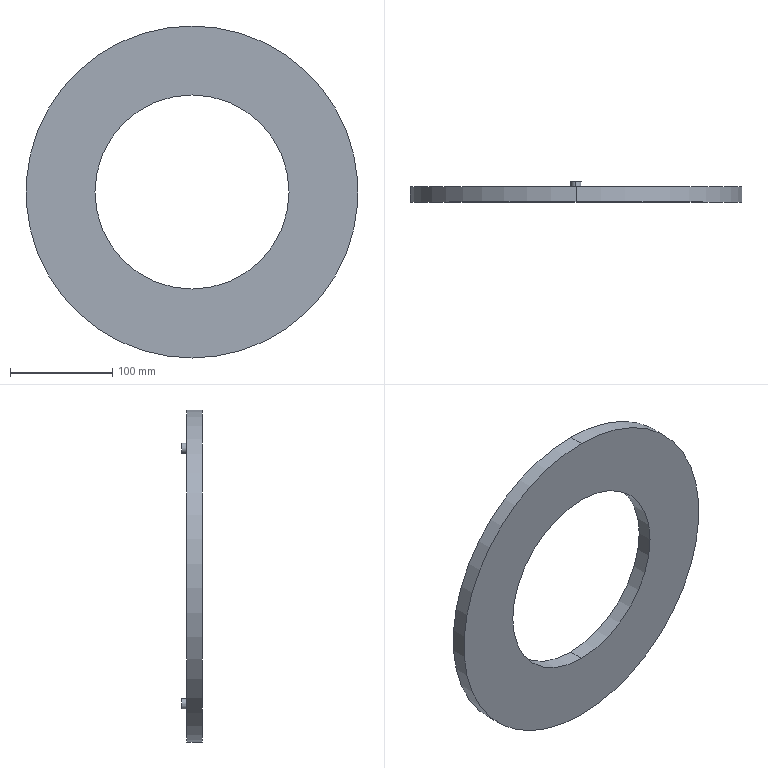Part | SolidWorks | features BaseBody 1 | 1 solid | 12 faces | box 325 x 20 x 325 mm | volume 819858 mm3 | cylinder 8 | plane 4 | commonest cylinder face diameters 10 x4 190 x2 325 x2
STEP:
#1=CARTESIAN_POINT('',(0.,20.,-120.));
#2=VERTEX_POINT('',#1);
#3=CARTESIAN_POINT('',(0.,20.,-130.));
#4=VERTEX_POINT('',#3);
#5=CARTESIAN_POINT('',(0.,20.,-125.));
#6=DIRECTION('',(0.,1.,0.));
#7=DIRECTION('',(0.,0.,1.));
#8=AXIS2_PLACEMENT_3D('',#5,#6,#7);
#9=CIRCLE('',#8,5.);
#10=EDGE_CURVE('',#2,#4,#9,.T.);
#11=ORIENTED_EDGE('',*,*,#10,.F.);
#12=CARTESIAN_POINT('',(0.,15.,-120.));
#13=VERTEX_POINT('',#12);
#14=CARTESIAN_POINT('',(0.,20.,-120.));
#15=DIRECTION('',(0.,-1.,0.));
#16=VECTOR('',#15,1000.);
#17=LINE('',#14,#16);
#18=EDGE_CURVE('',#2,#13,#17,.T.);
#19=ORIENTED_EDGE('',*,*,#18,.T.);
#20=CARTESIAN_POINT('',(0.,15.,-130.));
#21=VERTEX_POINT('',#20);
#22=CARTESIAN_POINT('',(0.,15.,-125.));
#23=DIRECTION('',(0.,1.,0.));
#24=DIRECTION('',(0.,0.,1.));
#25=AXIS2_PLACEMENT_3D('',#22,#23,#24);
#26=CIRCLE('',#25,5.);
#27=EDGE_CURVE('',#13,#21,#26,.T.);
#28=ORIENTED_EDGE('',*,*,#27,.T.);
#29=CARTESIAN_POINT('',(0.,20.,-130.));
#30=DIRECTION('',(0.,-1.,0.));
#31=VECTOR('',#30,1000.);
#32=LINE('',#29,#31);
#33=EDGE_CURVE('',#4,#21,#32,.T.);
#34=ORIENTED_EDGE('',*,*,#33,.F.);
#35=EDGE_LOOP('',(#11,#19,#28,#34));
#36=FACE_OUTER_BOUND('',#35,.T.);
#37=CARTESIAN_POINT('',(0.,20.,-125.));
#38=DIRECTION('',(0.,-1.,0.));
#39=DIRECTION('',(0.,0.,-1.));
#40=AXIS2_PLACEMENT_3D('',#37,#38,#39);
#41=CYLINDRICAL_SURFACE('',#40,5.);
#42=ADVANCED_FACE('',(#36),#41,.T.);
#43=CARTESIAN_POINT('',(0.,20.,130.));
#44=VERTEX_POINT('',#43);
#45=CARTESIAN_POINT('',(0.,20.,120.));
#46=VERTEX_POINT('',#45);
#47=CARTESIAN_POINT('',(0.,20.,125.));
#48=DIRECTION('',(0.,1.,0.));
#49=DIRECTION('',(0.,0.,1.));
#50=AXIS2_PLACEMENT_3D('',#47,#48,#49);
#51=CIRCLE('',#50,5.);
#52=EDGE_CURVE('',#44,#46,#51,.T.);
#53=ORIENTED_EDGE('',*,*,#52,.F.);
#54=CARTESIAN_POINT('',(0.,15.,130.));
#55=VERTEX_POINT('',#54);
#56=CARTESIAN_POINT('',(0.,20.,130.));
#57=DIRECTION('',(0.,-1.,0.));
#58=VECTOR('',#57,1000.);
#59=LINE('',#56,#58);
#60=EDGE_CURVE('',#44,#55,#59,.T.);
#61=ORIENTED_EDGE('',*,*,#60,.T.);
#62=CARTESIAN_POINT('',(0.,15.,120.));
#63=VERTEX_POINT('',#62);
#64=CARTESIAN_POINT('',(0.,15.,125.));
#65=DIRECTION('',(0.,1.,0.));
#66=DIRECTION('',(0.,0.,1.));
#67=AXIS2_PLACEMENT_3D('',#64,#65,#66);
#68=CIRCLE('',#67,5.);
#69=EDGE_CURVE('',#55,#63,#68,.T.);
#70=ORIENTED_EDGE('',*,*,#69,.T.);
#71=CARTESIAN_POINT('',(0.,20.,120.));
#72=DIRECTION('',(0.,-1.,0.));
#73=VECTOR('',#72,1000.);
#74=LINE('',#71,#73);
#75=EDGE_CURVE('',#46,#63,#74,.T.);
#76=ORIENTED_EDGE('',*,*,#75,.F.);
#77=EDGE_LOOP('',(#53,#61,#70,#76));
#78=FACE_OUTER_BOUND('',#77,.T.);
#79=CARTESIAN_POINT('',(0.,20.,125.));
#80=DIRECTION('',(0.,-1.,0.));
#81=DIRECTION('',(0.,0.,-1.));
#82=AXIS2_PLACEMENT_3D('',#79,#80,#81);
#83=CYLINDRICAL_SURFACE('',#82,5.);
#84=ADVANCED_FACE('',(#78),#83,.T.);
#85=CARTESIAN_POINT('',(0.,0.,-95.));
#86=VERTEX_POINT('',#85);
#87=CARTESIAN_POINT('',(0.,0.,95.));
#88=VERTEX_POINT('',#87);
#89=CARTESIAN_POINT('',(0.,0.,0.));
#90=DIRECTION('',(0.,1.,0.));
#91=DIRECTION('',(0.,0.,1.));
#92=AXIS2_PLACEMENT_3D('',#89,#90,#91);
#93=CIRCLE('',#92,95.);
#94=EDGE_CURVE('',#86,#88,#93,.T.);
#95=ORIENTED_EDGE('',*,*,#94,.F.);
#96=CARTESIAN_POINT('',(0.,15.,-95.));
#97=VERTEX_POINT('',#96);
#98=CARTESIAN_POINT('',(0.,0.,-95.));
#99=DIRECTION('',(0.,1.,0.));
#100=VECTOR('',#99,1000.);
#101=LINE('',#98,#100);
#102=EDGE_CURVE('',#86,#97,#101,.T.);
#103=ORIENTED_EDGE('',*,*,#102,.T.);
#104=CARTESIAN_POINT('',(0.,15.,95.));
#105=VERTEX_POINT('',#104);
#106=CARTESIAN_POINT('',(0.,15.,0.));
#107=DIRECTION('',(0.,1.,0.));
#108=DIRECTION('',(0.,0.,1.));
#109=AXIS2_PLACEMENT_3D('',#106,#107,#108);
#110=CIRCLE('',#109,95.);
#111=EDGE_CURVE('',#97,#105,#110,.T.);
#112=ORIENTED_EDGE('',*,*,#111,.T.);
#113=CARTESIAN_POINT('',(0.,0.,95.));
#114=DIRECTION('',(0.,1.,0.));
#115=VECTOR('',#114,1000.);
#116=LINE('',#113,#115);
#117=EDGE_CURVE('',#88,#105,#116,.T.);
#118=ORIENTED_EDGE('',*,*,#117,.F.);
#119=EDGE_LOOP('',(#95,#103,#112,#118));
#120=FACE_OUTER_BOUND('',#119,.T.);
#121=CARTESIAN_POINT('',(0.,0.,0.));
#122=DIRECTION('',(0.,1.,0.));
#123=DIRECTION('',(0.,0.,1.));
#124=AXIS2_PLACEMENT_3D('',#121,#122,#123);
#125=CYLINDRICAL_SURFACE('',#124,95.);
#126=ADVANCED_FACE('',(#120),#125,.F.);
#127=CARTESIAN_POINT('',(0.,15.,162.5));
#128=VERTEX_POINT('',#127);
#129=CARTESIAN_POINT('',(0.,15.,-162.5));
#130=VERTEX_POINT('',#129);
#131=CARTESIAN_POINT('',(0.,15.,0.));
#132=DIRECTION('',(0.,1.,0.));
#133=DIRECTION('',(0.,0.,1.));
#134=AXIS2_PLACEMENT_3D('',#131,#132,#133);
#135=CIRCLE('',#134,162.5);
#136=EDGE_CURVE('',#128,#130,#135,.T.);
#137=ORIENTED_EDGE('',*,*,#136,.F.);
#138=CARTESIAN_POINT('',(0.,0.,162.5));
#139=VERTEX_POINT('',#138);
#140=CARTESIAN_POINT('',(0.,15.,162.5));
#141=DIRECTION('',(0.,-1.,0.));
#142=VECTOR('',#141,1000.);
#143=LINE('',#140,#142);
#144=EDGE_CURVE('',#128,#139,#143,.T.);
#145=ORIENTED_EDGE('',*,*,#144,.T.);
#146=CARTESIAN_POINT('',(0.,0.,-162.5));
#147=VERTEX_POINT('',#146);
#148=CARTESIAN_POINT('',(0.,0.,0.));
#149=DIRECTION('',(0.,1.,0.));
#150=DIRECTION('',(0.,0.,1.));
#151=AXIS2_PLACEMENT_3D('',#148,#149,#150);
#152=CIRCLE('',#151,162.5);
#153=EDGE_CURVE('',#139,#147,#152,.T.);
#154=ORIENTED_EDGE('',*,*,#153,.T.);
#155=CARTESIAN_POINT('',(0.,15.,-162.5));
#156=DIRECTION('',(0.,-1.,0.));
#157=VECTOR('',#156,1000.);
#158=LINE('',#155,#157);
#159=EDGE_CURVE('',#130,#147,#158,.T.);
#160=ORIENTED_EDGE('',*,*,#159,.F.);
#161=EDGE_LOOP('',(#137,#145,#154,#160));
#162=FACE_OUTER_BOUND('',#161,.T.);
#163=CARTESIAN_POINT('',(0.,15.,0.));
#164=DIRECTION('',(0.,-1.,0.));
#165=DIRECTION('',(0.,0.,-1.));
#166=AXIS2_PLACEMENT_3D('',#163,#164,#165);
#167=CYLINDRICAL_SURFACE('',#166,162.5);
#168=ADVANCED_FACE('',(#162),#167,.T.);
#169=ORIENTED_EDGE('',*,*,#144,.F.);
#170=CARTESIAN_POINT('',(0.,15.,0.));
#171=DIRECTION('',(0.,1.,0.));
#172=DIRECTION('',(0.,0.,1.));
#173=AXIS2_PLACEMENT_3D('',#170,#171,#172);
#174=CIRCLE('',#173,162.5);
#175=EDGE_CURVE('',#130,#128,#174,.T.);
#176=ORIENTED_EDGE('',*,*,#175,.F.);
#177=ORIENTED_EDGE('',*,*,#159,.T.);
#178=CARTESIAN_POINT('',(0.,0.,0.));
#179=DIRECTION('',(0.,1.,0.));
#180=DIRECTION('',(0.,0.,1.));
#181=AXIS2_PLACEMENT_3D('',#178,#179,#180);
#182=CIRCLE('',#181,162.5);
#183=EDGE_CURVE('',#147,#139,#182,.T.);
#184=ORIENTED_EDGE('',*,*,#183,.T.);
#185=EDGE_LOOP('',(#169,#176,#177,#184));
#186=FACE_OUTER_BOUND('',#185,.T.);
#187=CARTESIAN_POINT('',(0.,15.,0.));
#188=DIRECTION('',(0.,-1.,0.));
#189=DIRECTION('',(0.,0.,-1.));
#190=AXIS2_PLACEMENT_3D('',#187,#188,#189);
#191=CYLINDRICAL_SURFACE('',#190,162.5);
#192=ADVANCED_FACE('',(#186),#191,.T.);
#193=CARTESIAN_POINT('',(0.,15.,-125.));
#194=DIRECTION('',(0.,1.,0.));
#195=DIRECTION('',(0.,0.,1.));
#196=AXIS2_PLACEMENT_3D('',#193,#194,#195);
#197=CIRCLE('',#196,5.);
#198=EDGE_CURVE('',#21,#13,#197,.T.);
#199=ORIENTED_EDGE('',*,*,#198,.F.);
#200=ORIENTED_EDGE('',*,*,#27,.F.);
#201=EDGE_LOOP('',(#199,#200));
#202=FACE_BOUND('',#201,.T.);
#203=CARTESIAN_POINT('',(0.,15.,125.));
#204=DIRECTION('',(0.,1.,0.));
#205=DIRECTION('',(0.,0.,1.));
#206=AXIS2_PLACEMENT_3D('',#203,#204,#205);
#207=CIRCLE('',#206,5.);
#208=EDGE_CURVE('',#63,#55,#207,.T.);
#209=ORIENTED_EDGE('',*,*,#208,.F.);
#210=ORIENTED_EDGE('',*,*,#69,.F.);
#211=EDGE_LOOP('',(#209,#210));
#212=FACE_BOUND('',#211,.T.);
#213=CARTESIAN_POINT('',(0.,15.,0.));
#214=DIRECTION('',(0.,1.,0.));
#215=DIRECTION('',(0.,0.,1.));
#216=AXIS2_PLACEMENT_3D('',#213,#214,#215);
#217=CIRCLE('',#216,95.);
#218=EDGE_CURVE('',#105,#97,#217,.T.);
#219=ORIENTED_EDGE('',*,*,#218,.F.);
#220=ORIENTED_EDGE('',*,*,#111,.F.);
#221=EDGE_LOOP('',(#219,#220));
#222=FACE_BOUND('',#221,.T.);
#223=ORIENTED_EDGE('',*,*,#175,.T.);
#224=ORIENTED_EDGE('',*,*,#136,.T.);
#225=EDGE_LOOP('',(#223,#224));
#226=FACE_OUTER_BOUND('',#225,.T.);
#227=CARTESIAN_POINT('',(0.,15.,0.));
#228=DIRECTION('',(0.,1.,0.));
#229=DIRECTION('',(0.,0.,1.));
#230=AXIS2_PLACEMENT_3D('',#227,#228,#229);
#231=PLANE('',#230);
#232=ADVANCED_FACE('',(#202,#212,#222,#226),#231,.T.);
#233=CARTESIAN_POINT('',(0.,0.,0.));
#234=DIRECTION('',(0.,1.,0.));
#235=DIRECTION('',(0.,0.,1.));
#236=AXIS2_PLACEMENT_3D('',#233,#234,#235);
#237=CIRCLE('',#236,95.);
#238=EDGE_CURVE('',#88,#86,#237,.T.);
#239=ORIENTED_EDGE('',*,*,#238,.T.);
#240=ORIENTED_EDGE('',*,*,#94,.T.);
#241=EDGE_LOOP('',(#239,#240));
#242=FACE_BOUND('',#241,.T.);
#243=ORIENTED_EDGE('',*,*,#183,.F.);
#244=ORIENTED_EDGE('',*,*,#153,.F.);
#245=EDGE_LOOP('',(#243,#244));
#246=FACE_OUTER_BOUND('',#245,.T.);
#247=CARTESIAN_POINT('',(0.,0.,0.));
#248=DIRECTION('',(0.,1.,0.));
#249=DIRECTION('',(0.,0.,1.));
#250=AXIS2_PLACEMENT_3D('',#247,#248,#249);
#251=PLANE('',#250);
#252=ADVANCED_FACE('',(#242,#246),#251,.F.);
#253=ORIENTED_EDGE('',*,*,#102,.F.);
#254=ORIENTED_EDGE('',*,*,#238,.F.);
#255=ORIENTED_EDGE('',*,*,#117,.T.);
#256=ORIENTED_EDGE('',*,*,#218,.T.);
#257=EDGE_LOOP('',(#253,#254,#255,#256));
#258=FACE_OUTER_BOUND('',#257,.T.);
#259=CARTESIAN_POINT('',(0.,0.,0.));
#260=DIRECTION('',(0.,1.,0.));
#261=DIRECTION('',(0.,0.,1.));
#262=AXIS2_PLACEMENT_3D('',#259,#260,#261);
#263=CYLINDRICAL_SURFACE('',#262,95.);
#264=ADVANCED_FACE('',(#258),#263,.F.);
#265=ORIENTED_EDGE('',*,*,#60,.F.);
#266=CARTESIAN_POINT('',(0.,20.,125.));
#267=DIRECTION('',(0.,1.,0.));
#268=DIRECTION('',(0.,0.,1.));
#269=AXIS2_PLACEMENT_3D('',#266,#267,#268);
#270=CIRCLE('',#269,5.);
#271=EDGE_CURVE('',#46,#44,#270,.T.);
#272=ORIENTED_EDGE('',*,*,#271,.F.);
#273=ORIENTED_EDGE('',*,*,#75,.T.);
#274=ORIENTED_EDGE('',*,*,#208,.T.);
#275=EDGE_LOOP('',(#265,#272,#273,#274));
#276=FACE_OUTER_BOUND('',#275,.T.);
#277=CARTESIAN_POINT('',(0.,20.,125.));
#278=DIRECTION('',(0.,-1.,0.));
#279=DIRECTION('',(0.,0.,-1.));
#280=AXIS2_PLACEMENT_3D('',#277,#278,#279);
#281=CYLINDRICAL_SURFACE('',#280,5.);
#282=ADVANCED_FACE('',(#276),#281,.T.);
#283=ORIENTED_EDGE('',*,*,#271,.T.);
#284=ORIENTED_EDGE('',*,*,#52,.T.);
#285=EDGE_LOOP('',(#283,#284));
#286=FACE_OUTER_BOUND('',#285,.T.);
#287=CARTESIAN_POINT('',(0.,20.,125.));
#288=DIRECTION('',(0.,1.,0.));
#289=DIRECTION('',(0.,0.,1.));
#290=AXIS2_PLACEMENT_3D('',#287,#288,#289);
#291=PLANE('',#290);
#292=ADVANCED_FACE('',(#286),#291,.T.);
#293=ORIENTED_EDGE('',*,*,#18,.F.);
#294=CARTESIAN_POINT('',(0.,20.,-125.));
#295=DIRECTION('',(0.,1.,0.));
#296=DIRECTION('',(0.,0.,1.));
#297=AXIS2_PLACEMENT_3D('',#294,#295,#296);
#298=CIRCLE('',#297,5.);
#299=EDGE_CURVE('',#4,#2,#298,.T.);
#300=ORIENTED_EDGE('',*,*,#299,.F.);
#301=ORIENTED_EDGE('',*,*,#33,.T.);
#302=ORIENTED_EDGE('',*,*,#198,.T.);
#303=EDGE_LOOP('',(#293,#300,#301,#302));
#304=FACE_OUTER_BOUND('',#303,.T.);
#305=CARTESIAN_POINT('',(0.,20.,-125.));
#306=DIRECTION('',(0.,-1.,0.));
#307=DIRECTION('',(0.,0.,-1.));
#308=AXIS2_PLACEMENT_3D('',#305,#306,#307);
#309=CYLINDRICAL_SURFACE('',#308,5.);
#310=ADVANCED_FACE('',(#304),#309,.T.);
#311=ORIENTED_EDGE('',*,*,#299,.T.);
#312=ORIENTED_EDGE('',*,*,#10,.T.);
#313=EDGE_LOOP('',(#311,#312));
#314=FACE_OUTER_BOUND('',#313,.T.);
#315=CARTESIAN_POINT('',(0.,20.,-125.));
#316=DIRECTION('',(0.,1.,0.));
#317=DIRECTION('',(0.,0.,1.));
#318=AXIS2_PLACEMENT_3D('',#315,#316,#317);
#319=PLANE('',#318);
#320=ADVANCED_FACE('',(#314),#319,.T.);
#321=CLOSED_SHELL('',(#42,#84,#126,#168,#192,#232,#252,#264,#282,#292,#310,#320));
#322=MANIFOLD_SOLID_BREP('',#321);
#323=CARTESIAN_POINT('',(0.,0.,0.));
#324=DIRECTION('',(0.,0.,1.));
#325=DIRECTION('',(1.,0.,0.));
#326=AXIS2_PLACEMENT_3D('',#323,#324,#325);
#327=(LENGTH_UNIT()NAMED_UNIT(*)SI_UNIT(.MILLI.,.METRE.));
#328=UNCERTAINTY_MEASURE_WITH_UNIT(LENGTH_MEASURE(0.00001),#327,'','');
#329=(NAMED_UNIT(*)PLANE_ANGLE_UNIT()SI_UNIT($,.RADIAN.));
#330=(NAMED_UNIT(*)SI_UNIT($,.STERADIAN.)SOLID_ANGLE_UNIT());
#331=(GEOMETRIC_REPRESENTATION_CONTEXT(3)GLOBAL_UNCERTAINTY_ASSIGNED_CONTEXT((#328))GLOBAL_UNIT_ASSIGNED_CONTEXT((#327,#329,#330))REPRESENTATION_CONTEXT('',''));
#332=ADVANCED_BREP_SHAPE_REPRESENTATION('',(#322,#326),#331);